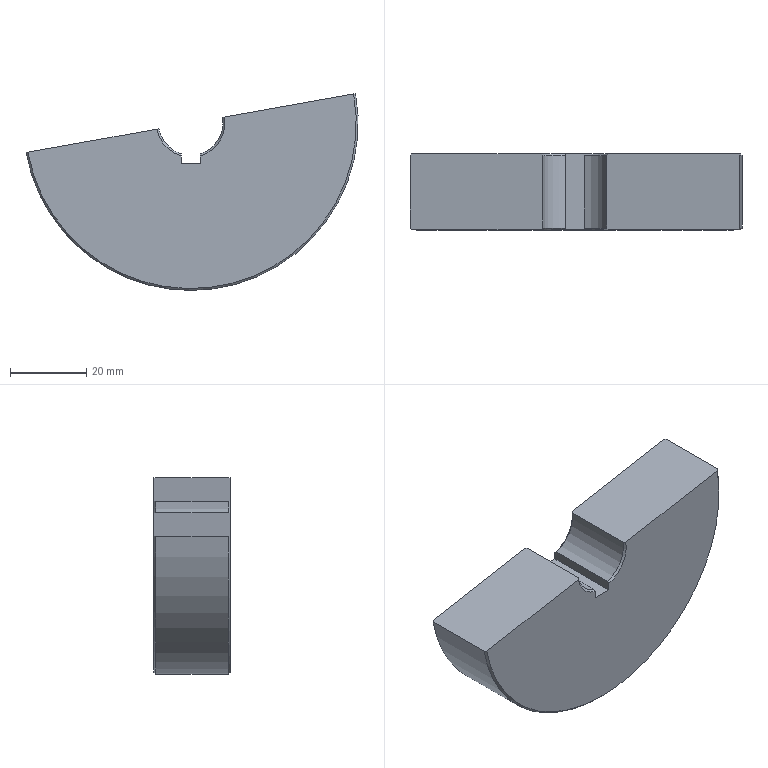Part | STEP file | Cuon T phu H01_6 | 1 solid | 18 faces | box 87.312 x 20 x 51.753 mm | volume 58287 mm3 | cone 7 | plane 7 | cylinder 4 | commonest cylinder face diameters 17 x2 88 x2